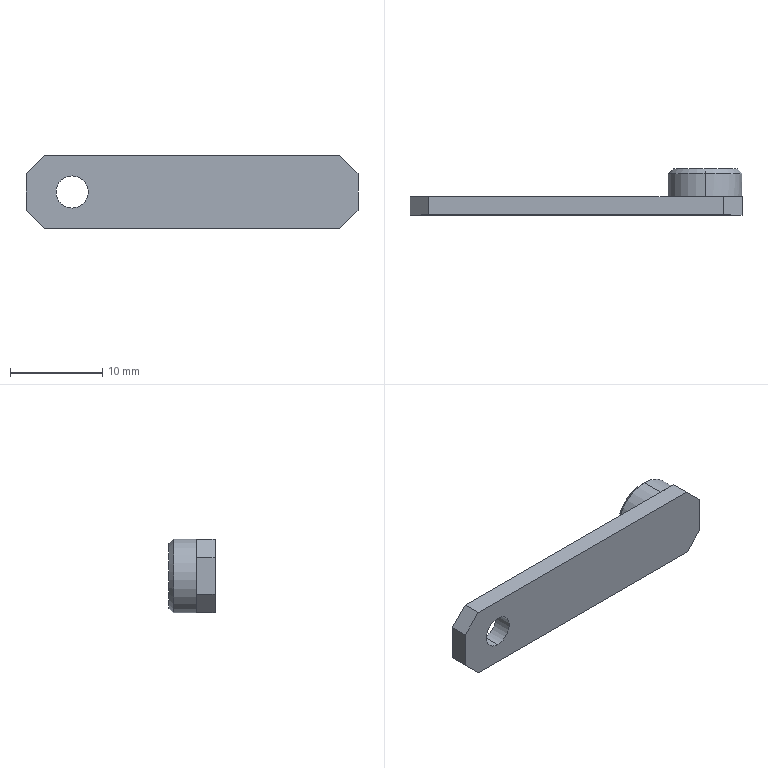Part | SolidWorks | features Chamfer 2, ICE 2, Extrusion 1 | 1 solid | 19 faces | box 36 x 5 x 8 mm | volume 688.543 mm3 | plane 13 | cylinder 4 | cone 2 | commonest cylinder face diameters 3.5 x2 8 x2
STEP:
#1=CARTESIAN_POINT('',(32.,5.,-0.5));
#2=VERTEX_POINT('',#1);
#3=CARTESIAN_POINT('',(32.,5.,-7.5));
#4=VERTEX_POINT('',#3);
#5=CARTESIAN_POINT('',(32.,5.,-4.));
#6=DIRECTION('',(0.,1.,0.));
#7=DIRECTION('',(0.,0.,1.));
#8=AXIS2_PLACEMENT_3D('',#5,#6,#7);
#9=CIRCLE('',#8,3.5);
#10=EDGE_CURVE('',#2,#4,#9,.T.);
#11=ORIENTED_EDGE('',*,*,#10,.F.);
#12=CARTESIAN_POINT('',(32.,4.5,0.));
#13=VERTEX_POINT('',#12);
#14=CARTESIAN_POINT('',(32.,5.,-0.5));
#15=DIRECTION('',(0.,-0.7071,0.7071));
#16=VECTOR('',#15,1000.);
#17=LINE('',#14,#16);
#18=EDGE_CURVE('',#2,#13,#17,.T.);
#19=ORIENTED_EDGE('',*,*,#18,.T.);
#20=CARTESIAN_POINT('',(32.,4.5,-8.));
#21=VERTEX_POINT('',#20);
#22=CARTESIAN_POINT('',(32.,4.5,-4.));
#23=DIRECTION('',(0.,-1.,0.));
#24=DIRECTION('',(0.,0.,1.));
#25=AXIS2_PLACEMENT_3D('',#22,#23,#24);
#26=CIRCLE('',#25,4.);
#27=EDGE_CURVE('',#21,#13,#26,.T.);
#28=ORIENTED_EDGE('',*,*,#27,.F.);
#29=CARTESIAN_POINT('',(32.,5.,-7.5));
#30=DIRECTION('',(0.,-0.7071,-0.7071));
#31=VECTOR('',#30,1000.);
#32=LINE('',#29,#31);
#33=EDGE_CURVE('',#4,#21,#32,.T.);
#34=ORIENTED_EDGE('',*,*,#33,.F.);
#35=EDGE_LOOP('',(#11,#19,#28,#34));
#36=FACE_OUTER_BOUND('',#35,.T.);
#37=CARTESIAN_POINT('',(32.,5.,-4.));
#38=DIRECTION('',(0.,-1.,0.));
#39=DIRECTION('',(0.,0.,-1.));
#40=AXIS2_PLACEMENT_3D('',#37,#38,#39);
#41=CONICAL_SURFACE('',#40,3.5,0.7854);
#42=ADVANCED_FACE('',(#36),#41,.T.);
#43=ORIENTED_EDGE('',*,*,#27,.T.);
#44=CARTESIAN_POINT('',(32.,2.,0.));
#45=VERTEX_POINT('',#44);
#46=CARTESIAN_POINT('',(32.,5.,0.));
#47=DIRECTION('',(0.,-1.,0.));
#48=VECTOR('',#47,1000.);
#49=LINE('',#46,#48);
#50=EDGE_CURVE('',#13,#45,#49,.T.);
#51=ORIENTED_EDGE('',*,*,#50,.T.);
#52=CARTESIAN_POINT('',(36.,2.,-4.));
#53=VERTEX_POINT('',#52);
#54=CARTESIAN_POINT('',(32.,2.,-4.));
#55=DIRECTION('',(0.,1.,0.));
#56=DIRECTION('',(0.,0.,1.));
#57=AXIS2_PLACEMENT_3D('',#54,#55,#56);
#58=CIRCLE('',#57,4.);
#59=EDGE_CURVE('',#45,#53,#58,.T.);
#60=ORIENTED_EDGE('',*,*,#59,.T.);
#61=CARTESIAN_POINT('',(32.,2.,-8.));
#62=VERTEX_POINT('',#61);
#63=CARTESIAN_POINT('',(32.,2.,-4.));
#64=DIRECTION('',(0.,1.,0.));
#65=DIRECTION('',(0.,0.,1.));
#66=AXIS2_PLACEMENT_3D('',#63,#64,#65);
#67=CIRCLE('',#66,4.);
#68=EDGE_CURVE('',#53,#62,#67,.T.);
#69=ORIENTED_EDGE('',*,*,#68,.T.);
#70=CARTESIAN_POINT('',(32.,5.,-8.));
#71=DIRECTION('',(0.,-1.,0.));
#72=VECTOR('',#71,1000.);
#73=LINE('',#70,#72);
#74=EDGE_CURVE('',#21,#62,#73,.T.);
#75=ORIENTED_EDGE('',*,*,#74,.F.);
#76=EDGE_LOOP('',(#43,#51,#60,#69,#75));
#77=FACE_OUTER_BOUND('',#76,.T.);
#78=CARTESIAN_POINT('',(32.,5.,-4.));
#79=DIRECTION('',(0.,-1.,0.));
#80=DIRECTION('',(0.,0.,-1.));
#81=AXIS2_PLACEMENT_3D('',#78,#79,#80);
#82=CYLINDRICAL_SURFACE('',#81,4.);
#83=ADVANCED_FACE('',(#77),#82,.T.);
#84=CARTESIAN_POINT('',(5.,0.,-5.75));
#85=VERTEX_POINT('',#84);
#86=CARTESIAN_POINT('',(5.,0.,-2.25));
#87=VERTEX_POINT('',#86);
#88=CARTESIAN_POINT('',(5.,0.,-4.));
#89=DIRECTION('',(0.,1.,0.));
#90=DIRECTION('',(0.,0.,1.));
#91=AXIS2_PLACEMENT_3D('',#88,#89,#90);
#92=CIRCLE('',#91,1.75);
#93=EDGE_CURVE('',#85,#87,#92,.T.);
#94=ORIENTED_EDGE('',*,*,#93,.F.);
#95=CARTESIAN_POINT('',(5.,2.,-5.75));
#96=VERTEX_POINT('',#95);
#97=CARTESIAN_POINT('',(5.,0.,-5.75));
#98=DIRECTION('',(0.,1.,0.));
#99=VECTOR('',#98,1000.);
#100=LINE('',#97,#99);
#101=EDGE_CURVE('',#85,#96,#100,.T.);
#102=ORIENTED_EDGE('',*,*,#101,.T.);
#103=CARTESIAN_POINT('',(5.,2.,-2.25));
#104=VERTEX_POINT('',#103);
#105=CARTESIAN_POINT('',(5.,2.,-4.));
#106=DIRECTION('',(0.,1.,0.));
#107=DIRECTION('',(0.,0.,1.));
#108=AXIS2_PLACEMENT_3D('',#105,#106,#107);
#109=CIRCLE('',#108,1.75);
#110=EDGE_CURVE('',#96,#104,#109,.T.);
#111=ORIENTED_EDGE('',*,*,#110,.T.);
#112=CARTESIAN_POINT('',(5.,0.,-2.25));
#113=DIRECTION('',(0.,1.,0.));
#114=VECTOR('',#113,1000.);
#115=LINE('',#112,#114);
#116=EDGE_CURVE('',#87,#104,#115,.T.);
#117=ORIENTED_EDGE('',*,*,#116,.F.);
#118=EDGE_LOOP('',(#94,#102,#111,#117));
#119=FACE_OUTER_BOUND('',#118,.T.);
#120=CARTESIAN_POINT('',(5.,0.,-4.));
#121=DIRECTION('',(0.,1.,0.));
#122=DIRECTION('',(0.,0.,1.));
#123=AXIS2_PLACEMENT_3D('',#120,#121,#122);
#124=CYLINDRICAL_SURFACE('',#123,1.75);
#125=ADVANCED_FACE('',(#119),#124,.F.);
#126=CARTESIAN_POINT('',(34.,2.,0.));
#127=VERTEX_POINT('',#126);
#128=CARTESIAN_POINT('',(0.,2.,0.));
#129=DIRECTION('',(1.,0.,0.));
#130=VECTOR('',#129,1000.);
#131=LINE('',#128,#130);
#132=EDGE_CURVE('',#45,#127,#131,.T.);
#133=ORIENTED_EDGE('',*,*,#132,.T.);
#134=CARTESIAN_POINT('',(36.,2.,-2.));
#135=VERTEX_POINT('',#134);
#136=CARTESIAN_POINT('',(17.,2.,17.));
#137=DIRECTION('',(0.7071,0.,-0.7071));
#138=VECTOR('',#137,1000.);
#139=LINE('',#136,#138);
#140=EDGE_CURVE('',#127,#135,#139,.T.);
#141=ORIENTED_EDGE('',*,*,#140,.T.);
#142=CARTESIAN_POINT('',(36.,2.,-8.));
#143=DIRECTION('',(0.,0.,-1.));
#144=VECTOR('',#143,1000.);
#145=LINE('',#142,#144);
#146=EDGE_CURVE('',#135,#53,#145,.T.);
#147=ORIENTED_EDGE('',*,*,#146,.T.);
#148=ORIENTED_EDGE('',*,*,#59,.F.);
#149=EDGE_LOOP('',(#133,#141,#147,#148));
#150=FACE_OUTER_BOUND('',#149,.T.);
#151=CARTESIAN_POINT('',(0.,2.,0.));
#152=DIRECTION('',(0.,1.,0.));
#153=DIRECTION('',(0.,0.,1.));
#154=AXIS2_PLACEMENT_3D('',#151,#152,#153);
#155=PLANE('',#154);
#156=ADVANCED_FACE('',(#150),#155,.T.);
#157=CARTESIAN_POINT('',(36.,2.,-6.));
#158=VERTEX_POINT('',#157);
#159=CARTESIAN_POINT('',(36.,2.,-8.));
#160=DIRECTION('',(0.,0.,-1.));
#161=VECTOR('',#160,1000.);
#162=LINE('',#159,#161);
#163=EDGE_CURVE('',#53,#158,#162,.T.);
#164=ORIENTED_EDGE('',*,*,#163,.T.);
#165=CARTESIAN_POINT('',(34.,2.,-8.));
#166=VERTEX_POINT('',#165);
#167=CARTESIAN_POINT('',(21.,2.,-21.));
#168=DIRECTION('',(-0.7071,0.,-0.7071));
#169=VECTOR('',#168,1000.);
#170=LINE('',#167,#169);
#171=EDGE_CURVE('',#158,#166,#170,.T.);
#172=ORIENTED_EDGE('',*,*,#171,.T.);
#173=CARTESIAN_POINT('',(0.,2.,-8.));
#174=DIRECTION('',(-1.,0.,0.));
#175=VECTOR('',#174,1000.);
#176=LINE('',#173,#175);
#177=EDGE_CURVE('',#166,#62,#176,.T.);
#178=ORIENTED_EDGE('',*,*,#177,.T.);
#179=ORIENTED_EDGE('',*,*,#68,.F.);
#180=EDGE_LOOP('',(#164,#172,#178,#179));
#181=FACE_OUTER_BOUND('',#180,.T.);
#182=CARTESIAN_POINT('',(0.,2.,0.));
#183=DIRECTION('',(0.,1.,0.));
#184=DIRECTION('',(0.,0.,1.));
#185=AXIS2_PLACEMENT_3D('',#182,#183,#184);
#186=PLANE('',#185);
#187=ADVANCED_FACE('',(#181),#186,.T.);
#188=CARTESIAN_POINT('',(0.,0.,-6.));
#189=VERTEX_POINT('',#188);
#190=CARTESIAN_POINT('',(0.,0.,-2.));
#191=VERTEX_POINT('',#190);
#192=CARTESIAN_POINT('',(0.,0.,-8.));
#193=DIRECTION('',(0.,0.,1.));
#194=VECTOR('',#193,1000.);
#195=LINE('',#192,#194);
#196=EDGE_CURVE('',#189,#191,#195,.T.);
#197=ORIENTED_EDGE('',*,*,#196,.T.);
#198=CARTESIAN_POINT('',(0.,2.,-2.));
#199=VERTEX_POINT('',#198);
#200=CARTESIAN_POINT('',(0.,2.,-2.));
#201=DIRECTION('',(0.,1.,0.));
#202=VECTOR('',#201,1000.);
#203=LINE('',#200,#202);
#204=EDGE_CURVE('',#191,#199,#203,.T.);
#205=ORIENTED_EDGE('',*,*,#204,.T.);
#206=CARTESIAN_POINT('',(0.,2.,-6.));
#207=VERTEX_POINT('',#206);
#208=CARTESIAN_POINT('',(0.,2.,-8.));
#209=DIRECTION('',(0.,0.,1.));
#210=VECTOR('',#209,1000.);
#211=LINE('',#208,#210);
#212=EDGE_CURVE('',#207,#199,#211,.T.);
#213=ORIENTED_EDGE('',*,*,#212,.F.);
#214=CARTESIAN_POINT('',(0.,2.,-6.));
#215=DIRECTION('',(0.,-1.,0.));
#216=VECTOR('',#215,1000.);
#217=LINE('',#214,#216);
#218=EDGE_CURVE('',#207,#189,#217,.T.);
#219=ORIENTED_EDGE('',*,*,#218,.T.);
#220=EDGE_LOOP('',(#197,#205,#213,#219));
#221=FACE_OUTER_BOUND('',#220,.T.);
#222=CARTESIAN_POINT('',(0.,2.,-8.));
#223=DIRECTION('',(1.,0.,0.));
#224=DIRECTION('',(0.,0.,-1.));
#225=AXIS2_PLACEMENT_3D('',#222,#223,#224);
#226=PLANE('',#225);
#227=ADVANCED_FACE('',(#221),#226,.F.);
#228=CARTESIAN_POINT('',(2.,0.,0.));
#229=VERTEX_POINT('',#228);
#230=CARTESIAN_POINT('',(34.,0.,0.));
#231=VERTEX_POINT('',#230);
#232=CARTESIAN_POINT('',(0.,0.,0.));
#233=DIRECTION('',(1.,0.,0.));
#234=VECTOR('',#233,1000.);
#235=LINE('',#232,#234);
#236=EDGE_CURVE('',#229,#231,#235,.T.);
#237=ORIENTED_EDGE('',*,*,#236,.T.);
#238=CARTESIAN_POINT('',(34.,2.,0.));
#239=DIRECTION('',(0.,1.,0.));
#240=VECTOR('',#239,1000.);
#241=LINE('',#238,#240);
#242=EDGE_CURVE('',#231,#127,#241,.T.);
#243=ORIENTED_EDGE('',*,*,#242,.T.);
#244=ORIENTED_EDGE('',*,*,#132,.F.);
#245=CARTESIAN_POINT('',(2.,2.,0.));
#246=VERTEX_POINT('',#245);
#247=CARTESIAN_POINT('',(0.,2.,0.));
#248=DIRECTION('',(1.,0.,0.));
#249=VECTOR('',#248,1000.);
#250=LINE('',#247,#249);
#251=EDGE_CURVE('',#246,#45,#250,.T.);
#252=ORIENTED_EDGE('',*,*,#251,.F.);
#253=CARTESIAN_POINT('',(2.,2.,0.));
#254=DIRECTION('',(0.,-1.,0.));
#255=VECTOR('',#254,1000.);
#256=LINE('',#253,#255);
#257=EDGE_CURVE('',#246,#229,#256,.T.);
#258=ORIENTED_EDGE('',*,*,#257,.T.);
#259=EDGE_LOOP('',(#237,#243,#244,#252,#258));
#260=FACE_OUTER_BOUND('',#259,.T.);
#261=CARTESIAN_POINT('',(0.,2.,0.));
#262=DIRECTION('',(0.,0.,-1.));
#263=DIRECTION('',(-1.,0.,0.));
#264=AXIS2_PLACEMENT_3D('',#261,#262,#263);
#265=PLANE('',#264);
#266=ADVANCED_FACE('',(#260),#265,.F.);
#267=CARTESIAN_POINT('',(36.,0.,-2.));
#268=VERTEX_POINT('',#267);
#269=CARTESIAN_POINT('',(36.,0.,-6.));
#270=VERTEX_POINT('',#269);
#271=CARTESIAN_POINT('',(36.,0.,-8.));
#272=DIRECTION('',(0.,0.,-1.));
#273=VECTOR('',#272,1000.);
#274=LINE('',#271,#273);
#275=EDGE_CURVE('',#268,#270,#274,.T.);
#276=ORIENTED_EDGE('',*,*,#275,.T.);
#277=CARTESIAN_POINT('',(36.,2.,-6.));
#278=DIRECTION('',(0.,1.,0.));
#279=VECTOR('',#278,1000.);
#280=LINE('',#277,#279);
#281=EDGE_CURVE('',#270,#158,#280,.T.);
#282=ORIENTED_EDGE('',*,*,#281,.T.);
#283=ORIENTED_EDGE('',*,*,#163,.F.);
#284=ORIENTED_EDGE('',*,*,#146,.F.);
#285=CARTESIAN_POINT('',(36.,2.,-2.));
#286=DIRECTION('',(0.,-1.,0.));
#287=VECTOR('',#286,1000.);
#288=LINE('',#285,#287);
#289=EDGE_CURVE('',#135,#268,#288,.T.);
#290=ORIENTED_EDGE('',*,*,#289,.T.);
#291=EDGE_LOOP('',(#276,#282,#283,#284,#290));
#292=FACE_OUTER_BOUND('',#291,.T.);
#293=CARTESIAN_POINT('',(36.,2.,-8.));
#294=DIRECTION('',(-1.,0.,0.));
#295=DIRECTION('',(0.,0.,1.));
#296=AXIS2_PLACEMENT_3D('',#293,#294,#295);
#297=PLANE('',#296);
#298=ADVANCED_FACE('',(#292),#297,.F.);
#299=ORIENTED_EDGE('',*,*,#177,.F.);
#300=CARTESIAN_POINT('',(34.,0.,-8.));
#301=VERTEX_POINT('',#300);
#302=CARTESIAN_POINT('',(34.,2.,-8.));
#303=DIRECTION('',(0.,-1.,0.));
#304=VECTOR('',#303,1000.);
#305=LINE('',#302,#304);
#306=EDGE_CURVE('',#166,#301,#305,.T.);
#307=ORIENTED_EDGE('',*,*,#306,.T.);
#308=CARTESIAN_POINT('',(2.,0.,-8.));
#309=VERTEX_POINT('',#308);
#310=CARTESIAN_POINT('',(0.,0.,-8.));
#311=DIRECTION('',(-1.,0.,0.));
#312=VECTOR('',#311,1000.);
#313=LINE('',#310,#312);
#314=EDGE_CURVE('',#301,#309,#313,.T.);
#315=ORIENTED_EDGE('',*,*,#314,.T.);
#316=CARTESIAN_POINT('',(2.,2.,-8.));
#317=VERTEX_POINT('',#316);
#318=CARTESIAN_POINT('',(2.,2.,-8.));
#319=DIRECTION('',(0.,1.,0.));
#320=VECTOR('',#319,1000.);
#321=LINE('',#318,#320);
#322=EDGE_CURVE('',#309,#317,#321,.T.);
#323=ORIENTED_EDGE('',*,*,#322,.T.);
#324=CARTESIAN_POINT('',(0.,2.,-8.));
#325=DIRECTION('',(-1.,0.,0.));
#326=VECTOR('',#325,1000.);
#327=LINE('',#324,#326);
#328=EDGE_CURVE('',#62,#317,#327,.T.);
#329=ORIENTED_EDGE('',*,*,#328,.F.);
#330=EDGE_LOOP('',(#299,#307,#315,#323,#329));
#331=FACE_OUTER_BOUND('',#330,.T.);
#332=CARTESIAN_POINT('',(0.,2.,-8.));
#333=DIRECTION('',(0.,0.,1.));
#334=DIRECTION('',(1.,0.,0.));
#335=AXIS2_PLACEMENT_3D('',#332,#333,#334);
#336=PLANE('',#335);
#337=ADVANCED_FACE('',(#331),#336,.F.);
#338=ORIENTED_EDGE('',*,*,#212,.T.);
#339=CARTESIAN_POINT('',(1.,2.,-1.));
#340=DIRECTION('',(0.7071,0.,0.7071));
#341=VECTOR('',#340,1000.);
#342=LINE('',#339,#341);
#343=EDGE_CURVE('',#199,#246,#342,.T.);
#344=ORIENTED_EDGE('',*,*,#343,.T.);
#345=ORIENTED_EDGE('',*,*,#251,.T.);
#346=CARTESIAN_POINT('',(32.,2.,-4.));
#347=DIRECTION('',(0.,1.,0.));
#348=DIRECTION('',(0.,0.,1.));
#349=AXIS2_PLACEMENT_3D('',#346,#347,#348);
#350=CIRCLE('',#349,4.);
#351=EDGE_CURVE('',#62,#45,#350,.T.);
#352=ORIENTED_EDGE('',*,*,#351,.F.);
#353=ORIENTED_EDGE('',*,*,#328,.T.);
#354=CARTESIAN_POINT('',(-3.,2.,-3.));
#355=DIRECTION('',(-0.7071,0.,0.7071));
#356=VECTOR('',#355,1000.);
#357=LINE('',#354,#356);
#358=EDGE_CURVE('',#317,#207,#357,.T.);
#359=ORIENTED_EDGE('',*,*,#358,.T.);
#360=EDGE_LOOP('',(#338,#344,#345,#352,#353,#359));
#361=FACE_OUTER_BOUND('',#360,.T.);
#362=CARTESIAN_POINT('',(5.,2.,-4.));
#363=DIRECTION('',(0.,1.,0.));
#364=DIRECTION('',(0.,0.,1.));
#365=AXIS2_PLACEMENT_3D('',#362,#363,#364);
#366=CIRCLE('',#365,1.75);
#367=EDGE_CURVE('',#104,#96,#366,.T.);
#368=ORIENTED_EDGE('',*,*,#367,.F.);
#369=ORIENTED_EDGE('',*,*,#110,.F.);
#370=EDGE_LOOP('',(#368,#369));
#371=FACE_BOUND('',#370,.T.);
#372=CARTESIAN_POINT('',(0.,2.,0.));
#373=DIRECTION('',(0.,1.,0.));
#374=DIRECTION('',(0.,0.,1.));
#375=AXIS2_PLACEMENT_3D('',#372,#373,#374);
#376=PLANE('',#375);
#377=ADVANCED_FACE('',(#361,#371),#376,.T.);
#378=CARTESIAN_POINT('',(5.,0.,-4.));
#379=DIRECTION('',(0.,1.,0.));
#380=DIRECTION('',(0.,0.,1.));
#381=AXIS2_PLACEMENT_3D('',#378,#379,#380);
#382=CIRCLE('',#381,1.75);
#383=EDGE_CURVE('',#87,#85,#382,.T.);
#384=ORIENTED_EDGE('',*,*,#383,.T.);
#385=ORIENTED_EDGE('',*,*,#93,.T.);
#386=EDGE_LOOP('',(#384,#385));
#387=FACE_BOUND('',#386,.T.);
#388=ORIENTED_EDGE('',*,*,#314,.F.);
#389=CARTESIAN_POINT('',(34.,0.,-8.));
#390=DIRECTION('',(0.7071,0.,0.7071));
#391=VECTOR('',#390,1000.);
#392=LINE('',#389,#391);
#393=EDGE_CURVE('',#301,#270,#392,.T.);
#394=ORIENTED_EDGE('',*,*,#393,.T.);
#395=ORIENTED_EDGE('',*,*,#275,.F.);
#396=CARTESIAN_POINT('',(36.,0.,-2.));
#397=DIRECTION('',(-0.7071,0.,0.7071));
#398=VECTOR('',#397,1000.);
#399=LINE('',#396,#398);
#400=EDGE_CURVE('',#268,#231,#399,.T.);
#401=ORIENTED_EDGE('',*,*,#400,.T.);
#402=ORIENTED_EDGE('',*,*,#236,.F.);
#403=CARTESIAN_POINT('',(2.,0.,0.));
#404=DIRECTION('',(-0.7071,0.,-0.7071));
#405=VECTOR('',#404,1000.);
#406=LINE('',#403,#405);
#407=EDGE_CURVE('',#229,#191,#406,.T.);
#408=ORIENTED_EDGE('',*,*,#407,.T.);
#409=ORIENTED_EDGE('',*,*,#196,.F.);
#410=CARTESIAN_POINT('',(0.,0.,-6.));
#411=DIRECTION('',(0.7071,0.,-0.7071));
#412=VECTOR('',#411,1000.);
#413=LINE('',#410,#412);
#414=EDGE_CURVE('',#189,#309,#413,.T.);
#415=ORIENTED_EDGE('',*,*,#414,.T.);
#416=EDGE_LOOP('',(#388,#394,#395,#401,#402,#408,#409,#415));
#417=FACE_OUTER_BOUND('',#416,.T.);
#418=CARTESIAN_POINT('',(0.,0.,0.));
#419=DIRECTION('',(0.,1.,0.));
#420=DIRECTION('',(0.,0.,1.));
#421=AXIS2_PLACEMENT_3D('',#418,#419,#420);
#422=PLANE('',#421);
#423=ADVANCED_FACE('',(#387,#417),#422,.F.);
#424=ORIENTED_EDGE('',*,*,#101,.F.);
#425=ORIENTED_EDGE('',*,*,#383,.F.);
#426=ORIENTED_EDGE('',*,*,#116,.T.);
#427=ORIENTED_EDGE('',*,*,#367,.T.);
#428=EDGE_LOOP('',(#424,#425,#426,#427));
#429=FACE_OUTER_BOUND('',#428,.T.);
#430=CARTESIAN_POINT('',(5.,0.,-4.));
#431=DIRECTION('',(0.,1.,0.));
#432=DIRECTION('',(0.,0.,1.));
#433=AXIS2_PLACEMENT_3D('',#430,#431,#432);
#434=CYLINDRICAL_SURFACE('',#433,1.75);
#435=ADVANCED_FACE('',(#429),#434,.F.);
#436=ORIENTED_EDGE('',*,*,#50,.F.);
#437=CARTESIAN_POINT('',(32.,4.5,-4.));
#438=DIRECTION('',(0.,-1.,0.));
#439=DIRECTION('',(0.,0.,1.));
#440=AXIS2_PLACEMENT_3D('',#437,#438,#439);
#441=CIRCLE('',#440,4.);
#442=EDGE_CURVE('',#13,#21,#441,.T.);
#443=ORIENTED_EDGE('',*,*,#442,.T.);
#444=ORIENTED_EDGE('',*,*,#74,.T.);
#445=ORIENTED_EDGE('',*,*,#351,.T.);
#446=EDGE_LOOP('',(#436,#443,#444,#445));
#447=FACE_OUTER_BOUND('',#446,.T.);
#448=CARTESIAN_POINT('',(32.,5.,-4.));
#449=DIRECTION('',(0.,-1.,0.));
#450=DIRECTION('',(0.,0.,-1.));
#451=AXIS2_PLACEMENT_3D('',#448,#449,#450);
#452=CYLINDRICAL_SURFACE('',#451,4.);
#453=ADVANCED_FACE('',(#447),#452,.T.);
#454=CARTESIAN_POINT('',(32.,5.,-4.));
#455=DIRECTION('',(0.,1.,0.));
#456=DIRECTION('',(0.,0.,1.));
#457=AXIS2_PLACEMENT_3D('',#454,#455,#456);
#458=CIRCLE('',#457,3.5);
#459=EDGE_CURVE('',#4,#2,#458,.T.);
#460=ORIENTED_EDGE('',*,*,#459,.T.);
#461=ORIENTED_EDGE('',*,*,#10,.T.);
#462=EDGE_LOOP('',(#460,#461));
#463=FACE_OUTER_BOUND('',#462,.T.);
#464=CARTESIAN_POINT('',(32.,5.,-4.));
#465=DIRECTION('',(0.,1.,0.));
#466=DIRECTION('',(0.,0.,1.));
#467=AXIS2_PLACEMENT_3D('',#464,#465,#466);
#468=PLANE('',#467);
#469=ADVANCED_FACE('',(#463),#468,.T.);
#470=ORIENTED_EDGE('',*,*,#18,.F.);
#471=ORIENTED_EDGE('',*,*,#459,.F.);
#472=ORIENTED_EDGE('',*,*,#33,.T.);
#473=ORIENTED_EDGE('',*,*,#442,.F.);
#474=EDGE_LOOP('',(#470,#471,#472,#473));
#475=FACE_OUTER_BOUND('',#474,.T.);
#476=CARTESIAN_POINT('',(32.,5.,-4.));
#477=DIRECTION('',(0.,-1.,0.));
#478=DIRECTION('',(0.,0.,-1.));
#479=AXIS2_PLACEMENT_3D('',#476,#477,#478);
#480=CONICAL_SURFACE('',#479,3.5,0.7854);
#481=ADVANCED_FACE('',(#475),#480,.T.);
#482=ORIENTED_EDGE('',*,*,#171,.F.);
#483=ORIENTED_EDGE('',*,*,#281,.F.);
#484=ORIENTED_EDGE('',*,*,#393,.F.);
#485=ORIENTED_EDGE('',*,*,#306,.F.);
#486=EDGE_LOOP('',(#482,#483,#484,#485));
#487=FACE_OUTER_BOUND('',#486,.T.);
#488=CARTESIAN_POINT('',(34.,2.,-8.));
#489=DIRECTION('',(-0.7071,0.,0.7071));
#490=DIRECTION('',(0.,-1.,0.));
#491=AXIS2_PLACEMENT_3D('',#488,#489,#490);
#492=PLANE('',#491);
#493=ADVANCED_FACE('',(#487),#492,.F.);
#494=ORIENTED_EDGE('',*,*,#140,.F.);
#495=ORIENTED_EDGE('',*,*,#242,.F.);
#496=ORIENTED_EDGE('',*,*,#400,.F.);
#497=ORIENTED_EDGE('',*,*,#289,.F.);
#498=EDGE_LOOP('',(#494,#495,#496,#497));
#499=FACE_OUTER_BOUND('',#498,.T.);
#500=CARTESIAN_POINT('',(36.,2.,-2.));
#501=DIRECTION('',(-0.7071,0.,-0.7071));
#502=DIRECTION('',(0.,-1.,0.));
#503=AXIS2_PLACEMENT_3D('',#500,#501,#502);
#504=PLANE('',#503);
#505=ADVANCED_FACE('',(#499),#504,.F.);
#506=ORIENTED_EDGE('',*,*,#343,.F.);
#507=ORIENTED_EDGE('',*,*,#204,.F.);
#508=ORIENTED_EDGE('',*,*,#407,.F.);
#509=ORIENTED_EDGE('',*,*,#257,.F.);
#510=EDGE_LOOP('',(#506,#507,#508,#509));
#511=FACE_OUTER_BOUND('',#510,.T.);
#512=CARTESIAN_POINT('',(2.,2.,0.));
#513=DIRECTION('',(0.7071,0.,-0.7071));
#514=DIRECTION('',(0.,-1.,0.));
#515=AXIS2_PLACEMENT_3D('',#512,#513,#514);
#516=PLANE('',#515);
#517=ADVANCED_FACE('',(#511),#516,.F.);
#518=ORIENTED_EDGE('',*,*,#358,.F.);
#519=ORIENTED_EDGE('',*,*,#322,.F.);
#520=ORIENTED_EDGE('',*,*,#414,.F.);
#521=ORIENTED_EDGE('',*,*,#218,.F.);
#522=EDGE_LOOP('',(#518,#519,#520,#521));
#523=FACE_OUTER_BOUND('',#522,.T.);
#524=CARTESIAN_POINT('',(0.,2.,-6.));
#525=DIRECTION('',(0.7071,0.,0.7071));
#526=DIRECTION('',(0.,-1.,0.));
#527=AXIS2_PLACEMENT_3D('',#524,#525,#526);
#528=PLANE('',#527);
#529=ADVANCED_FACE('',(#523),#528,.F.);
#530=CLOSED_SHELL('',(#42,#83,#125,#156,#187,#227,#266,#298,#337,#377,#423,#435,#453,#469,#481,#493,#505,#517,#529));
#531=MANIFOLD_SOLID_BREP('',#530);
#532=CARTESIAN_POINT('',(0.,0.,0.));
#533=DIRECTION('',(0.,0.,1.));
#534=DIRECTION('',(1.,0.,0.));
#535=AXIS2_PLACEMENT_3D('',#532,#533,#534);
#536=(LENGTH_UNIT()NAMED_UNIT(*)SI_UNIT(.MILLI.,.METRE.));
#537=UNCERTAINTY_MEASURE_WITH_UNIT(LENGTH_MEASURE(0.00001),#536,'','');
#538=(NAMED_UNIT(*)PLANE_ANGLE_UNIT()SI_UNIT($,.RADIAN.));
#539=(NAMED_UNIT(*)SI_UNIT($,.STERADIAN.)SOLID_ANGLE_UNIT());
#540=(GEOMETRIC_REPRESENTATION_CONTEXT(3)GLOBAL_UNCERTAINTY_ASSIGNED_CONTEXT((#537))GLOBAL_UNIT_ASSIGNED_CONTEXT((#536,#538,#539))REPRESENTATION_CONTEXT('',''));
#541=ADVANCED_BREP_SHAPE_REPRESENTATION('',(#531,#535),#540);